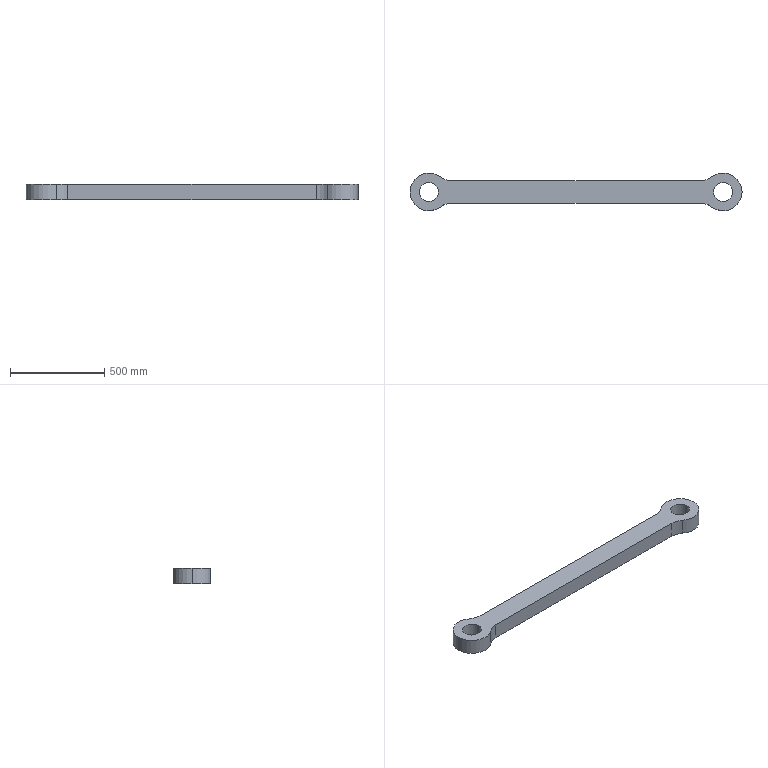Part | SolidWorks | features Extrusion 1 | 1 solid | 15 faces | box 1761 x 200 x 84 mm | volume 17816278 mm3 | cylinder 11 | plane 4 | commonest cylinder face diameters 200 x7 100 x4
STEP:
#1=CARTESIAN_POINT('',(773.42,0.,84.));
#2=VERTEX_POINT('',#1);
#3=CARTESIAN_POINT('',(873.42,0.,84.));
#4=VERTEX_POINT('',#3);
#5=CARTESIAN_POINT('',(823.42,0.,84.));
#6=DIRECTION('',(0.,0.,1.));
#7=DIRECTION('',(1.,0.,0.));
#8=AXIS2_PLACEMENT_3D('',#5,#6,#7);
#9=CIRCLE('',#8,50.);
#10=EDGE_CURVE('',#2,#4,#9,.T.);
#11=ORIENTED_EDGE('',*,*,#10,.T.);
#12=CARTESIAN_POINT('',(873.42,0.,0.));
#13=VERTEX_POINT('',#12);
#14=CARTESIAN_POINT('',(873.42,0.,84.));
#15=DIRECTION('',(0.,0.,-1.));
#16=VECTOR('',#15,1000.);
#17=LINE('',#14,#16);
#18=EDGE_CURVE('',#4,#13,#17,.T.);
#19=ORIENTED_EDGE('',*,*,#18,.T.);
#20=CARTESIAN_POINT('',(773.42,0.,0.));
#21=VERTEX_POINT('',#20);
#22=CARTESIAN_POINT('',(823.42,0.,0.));
#23=DIRECTION('',(0.,0.,1.));
#24=DIRECTION('',(1.,0.,0.));
#25=AXIS2_PLACEMENT_3D('',#22,#23,#24);
#26=CIRCLE('',#25,50.);
#27=EDGE_CURVE('',#21,#13,#26,.T.);
#28=ORIENTED_EDGE('',*,*,#27,.F.);
#29=CARTESIAN_POINT('',(773.42,0.,84.));
#30=DIRECTION('',(0.,0.,-1.));
#31=VECTOR('',#30,1000.);
#32=LINE('',#29,#31);
#33=EDGE_CURVE('',#2,#21,#32,.T.);
#34=ORIENTED_EDGE('',*,*,#33,.F.);
#35=EDGE_LOOP('',(#11,#19,#28,#34));
#36=FACE_OUTER_BOUND('',#35,.T.);
#37=CARTESIAN_POINT('',(823.42,0.,84.));
#38=DIRECTION('',(0.,0.,-1.));
#39=DIRECTION('',(-1.,0.,0.));
#40=AXIS2_PLACEMENT_3D('',#37,#38,#39);
#41=CYLINDRICAL_SURFACE('',#40,50.);
#42=ADVANCED_FACE('',(#36),#41,.F.);
#43=CARTESIAN_POINT('',(-787.58,0.,84.));
#44=VERTEX_POINT('',#43);
#45=CARTESIAN_POINT('',(-687.58,0.,84.));
#46=VERTEX_POINT('',#45);
#47=CARTESIAN_POINT('',(-737.58,0.,84.));
#48=DIRECTION('',(0.,0.,1.));
#49=DIRECTION('',(1.,0.,0.));
#50=AXIS2_PLACEMENT_3D('',#47,#48,#49);
#51=CIRCLE('',#50,50.);
#52=EDGE_CURVE('',#44,#46,#51,.T.);
#53=ORIENTED_EDGE('',*,*,#52,.T.);
#54=CARTESIAN_POINT('',(-687.58,0.,0.));
#55=VERTEX_POINT('',#54);
#56=CARTESIAN_POINT('',(-687.58,0.,84.));
#57=DIRECTION('',(0.,0.,-1.));
#58=VECTOR('',#57,1000.);
#59=LINE('',#56,#58);
#60=EDGE_CURVE('',#46,#55,#59,.T.);
#61=ORIENTED_EDGE('',*,*,#60,.T.);
#62=CARTESIAN_POINT('',(-787.58,0.,0.));
#63=VERTEX_POINT('',#62);
#64=CARTESIAN_POINT('',(-737.58,0.,0.));
#65=DIRECTION('',(0.,0.,1.));
#66=DIRECTION('',(1.,0.,0.));
#67=AXIS2_PLACEMENT_3D('',#64,#65,#66);
#68=CIRCLE('',#67,50.);
#69=EDGE_CURVE('',#63,#55,#68,.T.);
#70=ORIENTED_EDGE('',*,*,#69,.F.);
#71=CARTESIAN_POINT('',(-787.58,0.,84.));
#72=DIRECTION('',(0.,0.,-1.));
#73=VECTOR('',#72,1000.);
#74=LINE('',#71,#73);
#75=EDGE_CURVE('',#44,#63,#74,.T.);
#76=ORIENTED_EDGE('',*,*,#75,.F.);
#77=EDGE_LOOP('',(#53,#61,#70,#76));
#78=FACE_OUTER_BOUND('',#77,.T.);
#79=CARTESIAN_POINT('',(-737.58,0.,84.));
#80=DIRECTION('',(0.,0.,-1.));
#81=DIRECTION('',(-1.,0.,0.));
#82=AXIS2_PLACEMENT_3D('',#79,#80,#81);
#83=CYLINDRICAL_SURFACE('',#82,50.);
#84=ADVANCED_FACE('',(#78),#83,.F.);
#85=CARTESIAN_POINT('',(-837.58,0.,84.));
#86=VERTEX_POINT('',#85);
#87=CARTESIAN_POINT('',(-677.453,-79.905,84.));
#88=VERTEX_POINT('',#87);
#89=CARTESIAN_POINT('',(-737.58,0.,84.));
#90=DIRECTION('',(0.,0.,1.));
#91=DIRECTION('',(1.,0.,0.));
#92=AXIS2_PLACEMENT_3D('',#89,#90,#91);
#93=CIRCLE('',#92,100.);
#94=EDGE_CURVE('',#86,#88,#93,.T.);
#95=ORIENTED_EDGE('',*,*,#94,.F.);
#96=CARTESIAN_POINT('',(-837.58,0.,0.));
#97=VERTEX_POINT('',#96);
#98=CARTESIAN_POINT('',(-837.58,0.,84.));
#99=DIRECTION('',(0.,0.,-1.));
#100=VECTOR('',#99,1000.);
#101=LINE('',#98,#100);
#102=EDGE_CURVE('',#86,#97,#101,.T.);
#103=ORIENTED_EDGE('',*,*,#102,.T.);
#104=CARTESIAN_POINT('',(-677.453,-79.905,0.));
#105=VERTEX_POINT('',#104);
#106=CARTESIAN_POINT('',(-737.58,0.,0.));
#107=DIRECTION('',(0.,0.,1.));
#108=DIRECTION('',(1.,0.,0.));
#109=AXIS2_PLACEMENT_3D('',#106,#107,#108);
#110=CIRCLE('',#109,100.);
#111=EDGE_CURVE('',#97,#105,#110,.T.);
#112=ORIENTED_EDGE('',*,*,#111,.T.);
#113=CARTESIAN_POINT('',(-677.453,-79.905,84.));
#114=DIRECTION('',(0.,0.,-1.));
#115=VECTOR('',#114,1000.);
#116=LINE('',#113,#115);
#117=EDGE_CURVE('',#88,#105,#116,.T.);
#118=ORIENTED_EDGE('',*,*,#117,.F.);
#119=EDGE_LOOP('',(#95,#103,#112,#118));
#120=FACE_OUTER_BOUND('',#119,.T.);
#121=CARTESIAN_POINT('',(-737.58,0.,84.));
#122=DIRECTION('',(0.,0.,-1.));
#123=DIRECTION('',(-1.,0.,0.));
#124=AXIS2_PLACEMENT_3D('',#121,#122,#123);
#125=CYLINDRICAL_SURFACE('',#124,100.);
#126=ADVANCED_FACE('',(#120),#125,.T.);
#127=CARTESIAN_POINT('',(-617.326,59.809,0.));
#128=VERTEX_POINT('',#127);
#129=CARTESIAN_POINT('',(703.166,59.809,0.));
#130=VERTEX_POINT('',#129);
#131=CARTESIAN_POINT('',(0.,59.809,0.));
#132=DIRECTION('',(1.,0.,0.));
#133=VECTOR('',#132,1000.);
#134=LINE('',#131,#133);
#135=EDGE_CURVE('',#128,#130,#134,.T.);
#136=ORIENTED_EDGE('',*,*,#135,.F.);
#137=CARTESIAN_POINT('',(-617.326,59.809,84.));
#138=VERTEX_POINT('',#137);
#139=CARTESIAN_POINT('',(-617.326,59.809,84.));
#140=DIRECTION('',(0.,0.,-1.));
#141=VECTOR('',#140,1000.);
#142=LINE('',#139,#141);
#143=EDGE_CURVE('',#138,#128,#142,.T.);
#144=ORIENTED_EDGE('',*,*,#143,.F.);
#145=CARTESIAN_POINT('',(703.166,59.809,84.));
#146=VERTEX_POINT('',#145);
#147=CARTESIAN_POINT('',(0.,59.809,84.));
#148=DIRECTION('',(1.,0.,0.));
#149=VECTOR('',#148,1000.);
#150=LINE('',#147,#149);
#151=EDGE_CURVE('',#138,#146,#150,.T.);
#152=ORIENTED_EDGE('',*,*,#151,.T.);
#153=CARTESIAN_POINT('',(703.166,59.809,84.));
#154=DIRECTION('',(0.,0.,-1.));
#155=VECTOR('',#154,1000.);
#156=LINE('',#153,#155);
#157=EDGE_CURVE('',#146,#130,#156,.T.);
#158=ORIENTED_EDGE('',*,*,#157,.T.);
#159=EDGE_LOOP('',(#136,#144,#152,#158));
#160=FACE_OUTER_BOUND('',#159,.T.);
#161=CARTESIAN_POINT('',(0.,59.809,84.));
#162=DIRECTION('',(0.,1.,0.));
#163=DIRECTION('',(0.,0.,1.));
#164=AXIS2_PLACEMENT_3D('',#161,#162,#163);
#165=PLANE('',#164);
#166=ADVANCED_FACE('',(#160),#165,.T.);
#167=CARTESIAN_POINT('',(-677.453,79.905,0.));
#168=VERTEX_POINT('',#167);
#169=CARTESIAN_POINT('',(-617.326,159.809,0.));
#170=DIRECTION('',(0.,0.,-1.));
#171=DIRECTION('',(1.,0.,0.));
#172=AXIS2_PLACEMENT_3D('',#169,#170,#171);
#173=CIRCLE('',#172,100.);
#174=EDGE_CURVE('',#128,#168,#173,.T.);
#175=ORIENTED_EDGE('',*,*,#174,.T.);
#176=CARTESIAN_POINT('',(-677.453,79.905,84.));
#177=VERTEX_POINT('',#176);
#178=CARTESIAN_POINT('',(-677.453,79.905,84.));
#179=DIRECTION('',(0.,0.,-1.));
#180=VECTOR('',#179,1000.);
#181=LINE('',#178,#180);
#182=EDGE_CURVE('',#177,#168,#181,.T.);
#183=ORIENTED_EDGE('',*,*,#182,.F.);
#184=CARTESIAN_POINT('',(-617.326,159.809,84.));
#185=DIRECTION('',(0.,0.,-1.));
#186=DIRECTION('',(1.,0.,0.));
#187=AXIS2_PLACEMENT_3D('',#184,#185,#186);
#188=CIRCLE('',#187,100.);
#189=EDGE_CURVE('',#138,#177,#188,.T.);
#190=ORIENTED_EDGE('',*,*,#189,.F.);
#191=ORIENTED_EDGE('',*,*,#143,.T.);
#192=EDGE_LOOP('',(#175,#183,#190,#191));
#193=FACE_OUTER_BOUND('',#192,.T.);
#194=CARTESIAN_POINT('',(-617.326,159.809,84.));
#195=DIRECTION('',(0.,0.,-1.));
#196=DIRECTION('',(-1.,0.,0.));
#197=AXIS2_PLACEMENT_3D('',#194,#195,#196);
#198=CYLINDRICAL_SURFACE('',#197,100.);
#199=ADVANCED_FACE('',(#193),#198,.F.);
#200=ORIENTED_EDGE('',*,*,#102,.F.);
#201=CARTESIAN_POINT('',(-737.58,0.,84.));
#202=DIRECTION('',(0.,0.,1.));
#203=DIRECTION('',(1.,0.,0.));
#204=AXIS2_PLACEMENT_3D('',#201,#202,#203);
#205=CIRCLE('',#204,100.);
#206=EDGE_CURVE('',#177,#86,#205,.T.);
#207=ORIENTED_EDGE('',*,*,#206,.F.);
#208=ORIENTED_EDGE('',*,*,#182,.T.);
#209=CARTESIAN_POINT('',(-737.58,0.,0.));
#210=DIRECTION('',(0.,0.,1.));
#211=DIRECTION('',(1.,0.,0.));
#212=AXIS2_PLACEMENT_3D('',#209,#210,#211);
#213=CIRCLE('',#212,100.);
#214=EDGE_CURVE('',#168,#97,#213,.T.);
#215=ORIENTED_EDGE('',*,*,#214,.T.);
#216=EDGE_LOOP('',(#200,#207,#208,#215));
#217=FACE_OUTER_BOUND('',#216,.T.);
#218=CARTESIAN_POINT('',(-737.58,0.,84.));
#219=DIRECTION('',(0.,0.,-1.));
#220=DIRECTION('',(-1.,0.,0.));
#221=AXIS2_PLACEMENT_3D('',#218,#219,#220);
#222=CYLINDRICAL_SURFACE('',#221,100.);
#223=ADVANCED_FACE('',(#217),#222,.T.);
#224=CARTESIAN_POINT('',(-617.326,-59.809,0.));
#225=VERTEX_POINT('',#224);
#226=CARTESIAN_POINT('',(-617.326,-159.809,0.));
#227=DIRECTION('',(0.,0.,1.));
#228=DIRECTION('',(1.,0.,0.));
#229=AXIS2_PLACEMENT_3D('',#226,#227,#228);
#230=CIRCLE('',#229,100.);
#231=EDGE_CURVE('',#225,#105,#230,.T.);
#232=ORIENTED_EDGE('',*,*,#231,.F.);
#233=CARTESIAN_POINT('',(-617.326,-59.809,84.));
#234=VERTEX_POINT('',#233);
#235=CARTESIAN_POINT('',(-617.326,-59.809,84.));
#236=DIRECTION('',(0.,0.,-1.));
#237=VECTOR('',#236,1000.);
#238=LINE('',#235,#237);
#239=EDGE_CURVE('',#234,#225,#238,.T.);
#240=ORIENTED_EDGE('',*,*,#239,.F.);
#241=CARTESIAN_POINT('',(-617.326,-159.809,84.));
#242=DIRECTION('',(0.,0.,1.));
#243=DIRECTION('',(1.,0.,0.));
#244=AXIS2_PLACEMENT_3D('',#241,#242,#243);
#245=CIRCLE('',#244,100.);
#246=EDGE_CURVE('',#234,#88,#245,.T.);
#247=ORIENTED_EDGE('',*,*,#246,.T.);
#248=ORIENTED_EDGE('',*,*,#117,.T.);
#249=EDGE_LOOP('',(#232,#240,#247,#248));
#250=FACE_OUTER_BOUND('',#249,.T.);
#251=CARTESIAN_POINT('',(-617.326,-159.809,84.));
#252=DIRECTION('',(0.,0.,-1.));
#253=DIRECTION('',(-1.,0.,0.));
#254=AXIS2_PLACEMENT_3D('',#251,#252,#253);
#255=CYLINDRICAL_SURFACE('',#254,100.);
#256=ADVANCED_FACE('',(#250),#255,.F.);
#257=CARTESIAN_POINT('',(703.166,-59.809,0.));
#258=VERTEX_POINT('',#257);
#259=CARTESIAN_POINT('',(0.,-59.809,0.));
#260=DIRECTION('',(1.,0.,0.));
#261=VECTOR('',#260,1000.);
#262=LINE('',#259,#261);
#263=EDGE_CURVE('',#225,#258,#262,.T.);
#264=ORIENTED_EDGE('',*,*,#263,.T.);
#265=CARTESIAN_POINT('',(703.166,-59.809,84.));
#266=VERTEX_POINT('',#265);
#267=CARTESIAN_POINT('',(703.166,-59.809,84.));
#268=DIRECTION('',(0.,0.,-1.));
#269=VECTOR('',#268,1000.);
#270=LINE('',#267,#269);
#271=EDGE_CURVE('',#266,#258,#270,.T.);
#272=ORIENTED_EDGE('',*,*,#271,.F.);
#273=CARTESIAN_POINT('',(0.,-59.809,84.));
#274=DIRECTION('',(1.,0.,0.));
#275=VECTOR('',#274,1000.);
#276=LINE('',#273,#275);
#277=EDGE_CURVE('',#234,#266,#276,.T.);
#278=ORIENTED_EDGE('',*,*,#277,.F.);
#279=ORIENTED_EDGE('',*,*,#239,.T.);
#280=EDGE_LOOP('',(#264,#272,#278,#279));
#281=FACE_OUTER_BOUND('',#280,.T.);
#282=CARTESIAN_POINT('',(0.,-59.809,84.));
#283=DIRECTION('',(0.,1.,0.));
#284=DIRECTION('',(0.,0.,1.));
#285=AXIS2_PLACEMENT_3D('',#282,#283,#284);
#286=PLANE('',#285);
#287=ADVANCED_FACE('',(#281),#286,.F.);
#288=CARTESIAN_POINT('',(763.293,-79.905,0.));
#289=VERTEX_POINT('',#288);
#290=CARTESIAN_POINT('',(703.166,-159.809,0.));
#291=DIRECTION('',(0.,0.,1.));
#292=DIRECTION('',(1.,0.,0.));
#293=AXIS2_PLACEMENT_3D('',#290,#291,#292);
#294=CIRCLE('',#293,100.);
#295=EDGE_CURVE('',#289,#258,#294,.T.);
#296=ORIENTED_EDGE('',*,*,#295,.F.);
#297=CARTESIAN_POINT('',(763.293,-79.905,84.));
#298=VERTEX_POINT('',#297);
#299=CARTESIAN_POINT('',(763.293,-79.905,84.));
#300=DIRECTION('',(0.,0.,-1.));
#301=VECTOR('',#300,1000.);
#302=LINE('',#299,#301);
#303=EDGE_CURVE('',#298,#289,#302,.T.);
#304=ORIENTED_EDGE('',*,*,#303,.F.);
#305=CARTESIAN_POINT('',(703.166,-159.809,84.));
#306=DIRECTION('',(0.,0.,1.));
#307=DIRECTION('',(1.,0.,0.));
#308=AXIS2_PLACEMENT_3D('',#305,#306,#307);
#309=CIRCLE('',#308,100.);
#310=EDGE_CURVE('',#298,#266,#309,.T.);
#311=ORIENTED_EDGE('',*,*,#310,.T.);
#312=ORIENTED_EDGE('',*,*,#271,.T.);
#313=EDGE_LOOP('',(#296,#304,#311,#312));
#314=FACE_OUTER_BOUND('',#313,.T.);
#315=CARTESIAN_POINT('',(703.166,-159.809,84.));
#316=DIRECTION('',(0.,0.,-1.));
#317=DIRECTION('',(-1.,0.,0.));
#318=AXIS2_PLACEMENT_3D('',#315,#316,#317);
#319=CYLINDRICAL_SURFACE('',#318,100.);
#320=ADVANCED_FACE('',(#314),#319,.F.);
#321=CARTESIAN_POINT('',(763.293,79.905,0.));
#322=VERTEX_POINT('',#321);
#323=CARTESIAN_POINT('',(823.42,0.,0.));
#324=DIRECTION('',(0.,0.,1.));
#325=DIRECTION('',(1.,0.,0.));
#326=AXIS2_PLACEMENT_3D('',#323,#324,#325);
#327=CIRCLE('',#326,100.);
#328=EDGE_CURVE('',#289,#322,#327,.T.);
#329=ORIENTED_EDGE('',*,*,#328,.T.);
#330=CARTESIAN_POINT('',(763.293,79.905,84.));
#331=VERTEX_POINT('',#330);
#332=CARTESIAN_POINT('',(763.293,79.905,84.));
#333=DIRECTION('',(0.,0.,-1.));
#334=VECTOR('',#333,1000.);
#335=LINE('',#332,#334);
#336=EDGE_CURVE('',#331,#322,#335,.T.);
#337=ORIENTED_EDGE('',*,*,#336,.F.);
#338=CARTESIAN_POINT('',(823.42,0.,84.));
#339=DIRECTION('',(0.,0.,1.));
#340=DIRECTION('',(1.,0.,0.));
#341=AXIS2_PLACEMENT_3D('',#338,#339,#340);
#342=CIRCLE('',#341,100.);
#343=EDGE_CURVE('',#298,#331,#342,.T.);
#344=ORIENTED_EDGE('',*,*,#343,.F.);
#345=ORIENTED_EDGE('',*,*,#303,.T.);
#346=EDGE_LOOP('',(#329,#337,#344,#345));
#347=FACE_OUTER_BOUND('',#346,.T.);
#348=CARTESIAN_POINT('',(823.42,0.,84.));
#349=DIRECTION('',(0.,0.,-1.));
#350=DIRECTION('',(-1.,0.,0.));
#351=AXIS2_PLACEMENT_3D('',#348,#349,#350);
#352=CYLINDRICAL_SURFACE('',#351,100.);
#353=ADVANCED_FACE('',(#347),#352,.T.);
#354=ORIENTED_EDGE('',*,*,#60,.F.);
#355=CARTESIAN_POINT('',(-737.58,0.,84.));
#356=DIRECTION('',(0.,0.,1.));
#357=DIRECTION('',(1.,0.,0.));
#358=AXIS2_PLACEMENT_3D('',#355,#356,#357);
#359=CIRCLE('',#358,50.);
#360=EDGE_CURVE('',#46,#44,#359,.T.);
#361=ORIENTED_EDGE('',*,*,#360,.T.);
#362=ORIENTED_EDGE('',*,*,#75,.T.);
#363=CARTESIAN_POINT('',(-737.58,0.,0.));
#364=DIRECTION('',(0.,0.,1.));
#365=DIRECTION('',(1.,0.,0.));
#366=AXIS2_PLACEMENT_3D('',#363,#364,#365);
#367=CIRCLE('',#366,50.);
#368=EDGE_CURVE('',#55,#63,#367,.T.);
#369=ORIENTED_EDGE('',*,*,#368,.F.);
#370=EDGE_LOOP('',(#354,#361,#362,#369));
#371=FACE_OUTER_BOUND('',#370,.T.);
#372=CARTESIAN_POINT('',(-737.58,0.,84.));
#373=DIRECTION('',(0.,0.,-1.));
#374=DIRECTION('',(-1.,0.,0.));
#375=AXIS2_PLACEMENT_3D('',#372,#373,#374);
#376=CYLINDRICAL_SURFACE('',#375,50.);
#377=ADVANCED_FACE('',(#371),#376,.F.);
#378=ORIENTED_EDGE('',*,*,#18,.F.);
#379=CARTESIAN_POINT('',(823.42,0.,84.));
#380=DIRECTION('',(0.,0.,1.));
#381=DIRECTION('',(1.,0.,0.));
#382=AXIS2_PLACEMENT_3D('',#379,#380,#381);
#383=CIRCLE('',#382,50.);
#384=EDGE_CURVE('',#4,#2,#383,.T.);
#385=ORIENTED_EDGE('',*,*,#384,.T.);
#386=ORIENTED_EDGE('',*,*,#33,.T.);
#387=CARTESIAN_POINT('',(823.42,0.,0.));
#388=DIRECTION('',(0.,0.,1.));
#389=DIRECTION('',(1.,0.,0.));
#390=AXIS2_PLACEMENT_3D('',#387,#388,#389);
#391=CIRCLE('',#390,50.);
#392=EDGE_CURVE('',#13,#21,#391,.T.);
#393=ORIENTED_EDGE('',*,*,#392,.F.);
#394=EDGE_LOOP('',(#378,#385,#386,#393));
#395=FACE_OUTER_BOUND('',#394,.T.);
#396=CARTESIAN_POINT('',(823.42,0.,84.));
#397=DIRECTION('',(0.,0.,-1.));
#398=DIRECTION('',(-1.,0.,0.));
#399=AXIS2_PLACEMENT_3D('',#396,#397,#398);
#400=CYLINDRICAL_SURFACE('',#399,50.);
#401=ADVANCED_FACE('',(#395),#400,.F.);
#402=CARTESIAN_POINT('',(703.166,159.809,0.));
#403=DIRECTION('',(0.,0.,1.));
#404=DIRECTION('',(1.,0.,0.));
#405=AXIS2_PLACEMENT_3D('',#402,#403,#404);
#406=CIRCLE('',#405,100.);
#407=EDGE_CURVE('',#130,#322,#406,.T.);
#408=ORIENTED_EDGE('',*,*,#407,.F.);
#409=ORIENTED_EDGE('',*,*,#157,.F.);
#410=CARTESIAN_POINT('',(703.166,159.809,84.));
#411=DIRECTION('',(0.,0.,1.));
#412=DIRECTION('',(1.,0.,0.));
#413=AXIS2_PLACEMENT_3D('',#410,#411,#412);
#414=CIRCLE('',#413,100.);
#415=EDGE_CURVE('',#146,#331,#414,.T.);
#416=ORIENTED_EDGE('',*,*,#415,.T.);
#417=ORIENTED_EDGE('',*,*,#336,.T.);
#418=EDGE_LOOP('',(#408,#409,#416,#417));
#419=FACE_OUTER_BOUND('',#418,.T.);
#420=CARTESIAN_POINT('',(703.166,159.809,84.));
#421=DIRECTION('',(0.,0.,-1.));
#422=DIRECTION('',(-1.,0.,0.));
#423=AXIS2_PLACEMENT_3D('',#420,#421,#422);
#424=CYLINDRICAL_SURFACE('',#423,100.);
#425=ADVANCED_FACE('',(#419),#424,.F.);
#426=ORIENTED_EDGE('',*,*,#10,.F.);
#427=ORIENTED_EDGE('',*,*,#384,.F.);
#428=EDGE_LOOP('',(#426,#427));
#429=FACE_BOUND('',#428,.T.);
#430=ORIENTED_EDGE('',*,*,#52,.F.);
#431=ORIENTED_EDGE('',*,*,#360,.F.);
#432=EDGE_LOOP('',(#430,#431));
#433=FACE_BOUND('',#432,.T.);
#434=ORIENTED_EDGE('',*,*,#151,.F.);
#435=ORIENTED_EDGE('',*,*,#189,.T.);
#436=ORIENTED_EDGE('',*,*,#206,.T.);
#437=ORIENTED_EDGE('',*,*,#94,.T.);
#438=ORIENTED_EDGE('',*,*,#246,.F.);
#439=ORIENTED_EDGE('',*,*,#277,.T.);
#440=ORIENTED_EDGE('',*,*,#310,.F.);
#441=ORIENTED_EDGE('',*,*,#343,.T.);
#442=ORIENTED_EDGE('',*,*,#415,.F.);
#443=EDGE_LOOP('',(#434,#435,#436,#437,#438,#439,#440,#441,#442));
#444=FACE_OUTER_BOUND('',#443,.T.);
#445=CARTESIAN_POINT('',(0.,0.,84.));
#446=DIRECTION('',(0.,0.,1.));
#447=DIRECTION('',(1.,0.,0.));
#448=AXIS2_PLACEMENT_3D('',#445,#446,#447);
#449=PLANE('',#448);
#450=ADVANCED_FACE('',(#429,#433,#444),#449,.T.);
#451=ORIENTED_EDGE('',*,*,#27,.T.);
#452=ORIENTED_EDGE('',*,*,#392,.T.);
#453=EDGE_LOOP('',(#451,#452));
#454=FACE_BOUND('',#453,.T.);
#455=ORIENTED_EDGE('',*,*,#69,.T.);
#456=ORIENTED_EDGE('',*,*,#368,.T.);
#457=EDGE_LOOP('',(#455,#456));
#458=FACE_BOUND('',#457,.T.);
#459=ORIENTED_EDGE('',*,*,#135,.T.);
#460=ORIENTED_EDGE('',*,*,#407,.T.);
#461=ORIENTED_EDGE('',*,*,#328,.F.);
#462=ORIENTED_EDGE('',*,*,#295,.T.);
#463=ORIENTED_EDGE('',*,*,#263,.F.);
#464=ORIENTED_EDGE('',*,*,#231,.T.);
#465=ORIENTED_EDGE('',*,*,#111,.F.);
#466=ORIENTED_EDGE('',*,*,#214,.F.);
#467=ORIENTED_EDGE('',*,*,#174,.F.);
#468=EDGE_LOOP('',(#459,#460,#461,#462,#463,#464,#465,#466,#467));
#469=FACE_OUTER_BOUND('',#468,.T.);
#470=CARTESIAN_POINT('',(0.,0.,0.));
#471=DIRECTION('',(0.,0.,1.));
#472=DIRECTION('',(1.,0.,0.));
#473=AXIS2_PLACEMENT_3D('',#470,#471,#472);
#474=PLANE('',#473);
#475=ADVANCED_FACE('',(#454,#458,#469),#474,.F.);
#476=CLOSED_SHELL('',(#42,#84,#126,#166,#199,#223,#256,#287,#320,#353,#377,#401,#425,#450,#475));
#477=MANIFOLD_SOLID_BREP('',#476);
#478=CARTESIAN_POINT('',(0.,0.,0.));
#479=DIRECTION('',(0.,0.,1.));
#480=DIRECTION('',(1.,0.,0.));
#481=AXIS2_PLACEMENT_3D('',#478,#479,#480);
#482=(LENGTH_UNIT()NAMED_UNIT(*)SI_UNIT(.MILLI.,.METRE.));
#483=UNCERTAINTY_MEASURE_WITH_UNIT(LENGTH_MEASURE(0.00001),#482,'','');
#484=(NAMED_UNIT(*)PLANE_ANGLE_UNIT()SI_UNIT($,.RADIAN.));
#485=(NAMED_UNIT(*)SI_UNIT($,.STERADIAN.)SOLID_ANGLE_UNIT());
#486=(GEOMETRIC_REPRESENTATION_CONTEXT(3)GLOBAL_UNCERTAINTY_ASSIGNED_CONTEXT((#483))GLOBAL_UNIT_ASSIGNED_CONTEXT((#482,#484,#485))REPRESENTATION_CONTEXT('',''));
#487=ADVANCED_BREP_SHAPE_REPRESENTATION('',(#477,#481),#486);